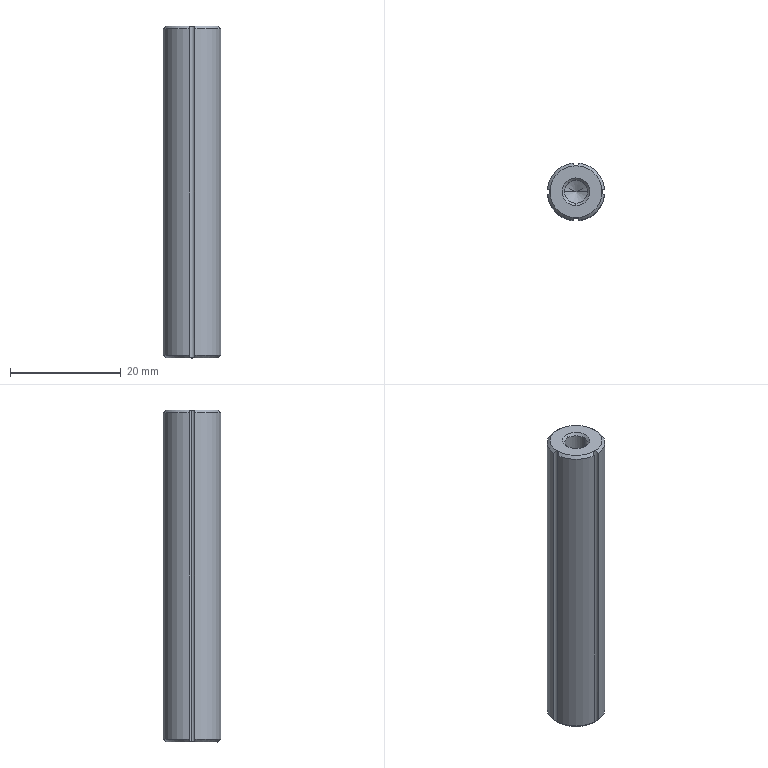Part | SolidWorks | features BaseBody 1 | 1 solid | 32 faces | box 10.348 x 10.348 x 60 mm | volume 4741 mm3 | cylinder 15 | cone 14 | plane 3 | commonest cylinder face diameters 1.04 x5 10.4 x4 2 x2 2.5 x2 4.134 x2
STEP:
#1=CARTESIAN_POINT('',(-4.68,0.,-30.));
#2=VERTEX_POINT('',#1);
#3=CARTESIAN_POINT('',(-4.698,0.1358,-30.));
#4=VERTEX_POINT('',#3);
#5=CARTESIAN_POINT('',(-5.2,0.,-30.));
#6=DIRECTION('',(0.,0.,1.));
#7=DIRECTION('',(1.,0.,0.));
#8=AXIS2_PLACEMENT_3D('',#5,#6,#7);
#9=CIRCLE('',#8,0.52);
#10=EDGE_CURVE('',#2,#4,#9,.T.);
#11=ORIENTED_EDGE('',*,*,#10,.F.);
#12=CARTESIAN_POINT('',(-4.68,0.,30.));
#13=VERTEX_POINT('',#12);
#14=CARTESIAN_POINT('',(-4.68,0.,30.));
#15=DIRECTION('',(0.,0.,1.));
#16=VECTOR('',#15,1000.);
#17=LINE('',#14,#16);
#18=EDGE_CURVE('',#2,#13,#17,.T.);
#19=ORIENTED_EDGE('',*,*,#18,.T.);
#20=CARTESIAN_POINT('',(-4.698,0.1358,30.));
#21=VERTEX_POINT('',#20);
#22=CARTESIAN_POINT('',(-5.2,0.,30.));
#23=DIRECTION('',(0.,0.,-1.));
#24=DIRECTION('',(1.,0.,0.));
#25=AXIS2_PLACEMENT_3D('',#22,#23,#24);
#26=CIRCLE('',#25,0.52);
#27=EDGE_CURVE('',#21,#13,#26,.T.);
#28=ORIENTED_EDGE('',*,*,#27,.F.);
#29=CARTESIAN_POINT('',(-5.174,0.5193,29.5));
#30=VERTEX_POINT('',#29);
#31=CARTESIAN_POINT('',(-5.174,0.5193,29.5));
#32=CARTESIAN_POINT('',(-5.076,0.5144,29.598));
#33=CARTESIAN_POINT('',(-4.981,0.483,29.696));
#34=CARTESIAN_POINT('',(-4.853,0.3908,29.831));
#35=CARTESIAN_POINT('',(-4.813,0.3523,29.874));
#36=CARTESIAN_POINT('',(-4.744,0.2574,29.949));
#37=CARTESIAN_POINT('',(-4.716,0.2008,29.981));
#38=CARTESIAN_POINT('',(-4.698,0.1358,30.));
#39=B_SPLINE_CURVE_WITH_KNOTS('',3,(#31,#32,#33,#34,#35,#36,#37,#38),.UNSPECIFIED.,.F.,.F.,(4,2,2,4),(0.,0.0004119,0.0006179,0.0008238),.UNSPECIFIED.);
#40=EDGE_CURVE('',#30,#21,#39,.T.);
#41=ORIENTED_EDGE('',*,*,#40,.F.);
#42=CARTESIAN_POINT('',(-5.174,0.5193,-29.5));
#43=VERTEX_POINT('',#42);
#44=CARTESIAN_POINT('',(-5.174,0.5193,0.));
#45=DIRECTION('',(0.,0.,1.));
#46=VECTOR('',#45,1000.);
#47=LINE('',#44,#46);
#48=EDGE_CURVE('',#43,#30,#47,.T.);
#49=ORIENTED_EDGE('',*,*,#48,.F.);
#50=CARTESIAN_POINT('',(-4.698,0.1358,-30.));
#51=CARTESIAN_POINT('',(-4.716,0.201,-29.98));
#52=CARTESIAN_POINT('',(-4.744,0.257,-29.949));
#53=CARTESIAN_POINT('',(-4.813,0.3519,-29.875));
#54=CARTESIAN_POINT('',(-4.852,0.3903,-29.832));
#55=CARTESIAN_POINT('',(-4.98,0.483,-29.696));
#56=CARTESIAN_POINT('',(-5.076,0.5144,-29.598));
#57=CARTESIAN_POINT('',(-5.174,0.5193,-29.5));
#58=B_SPLINE_CURVE_WITH_KNOTS('',3,(#50,#51,#52,#53,#54,#55,#56,#57),.UNSPECIFIED.,.F.,.F.,(4,2,2,4),(0.,0.0002068,0.0004137,0.0008273),.UNSPECIFIED.);
#59=EDGE_CURVE('',#4,#43,#58,.T.);
#60=ORIENTED_EDGE('',*,*,#59,.F.);
#61=EDGE_LOOP('',(#11,#19,#28,#41,#49,#60));
#62=FACE_OUTER_BOUND('',#61,.T.);
#63=CARTESIAN_POINT('',(-5.2,0.,30.));
#64=DIRECTION('',(0.,0.,1.));
#65=DIRECTION('',(1.,0.,0.));
#66=AXIS2_PLACEMENT_3D('',#63,#64,#65);
#67=CYLINDRICAL_SURFACE('',#66,0.52);
#68=ADVANCED_FACE('',(#62),#67,.F.);
#69=CARTESIAN_POINT('',(1.25,2.5,-22.5));
#70=VERTEX_POINT('',#69);
#71=CARTESIAN_POINT('',(-1.25,2.5,-22.5));
#72=VERTEX_POINT('',#71);
#73=CARTESIAN_POINT('',(0.,2.5,-22.5));
#74=DIRECTION('',(0.,0.,-1.));
#75=DIRECTION('',(-1.,0.,0.));
#76=AXIS2_PLACEMENT_3D('',#73,#74,#75);
#77=CIRCLE('',#76,1.25);
#78=EDGE_CURVE('',#70,#72,#77,.T.);
#79=ORIENTED_EDGE('',*,*,#78,.F.);
#80=CARTESIAN_POINT('',(1.25,2.5,-30.));
#81=VERTEX_POINT('',#80);
#82=CARTESIAN_POINT('',(1.25,2.5,-30.));
#83=DIRECTION('',(0.,0.,-1.));
#84=VECTOR('',#83,1000.);
#85=LINE('',#82,#84);
#86=EDGE_CURVE('',#70,#81,#85,.T.);
#87=ORIENTED_EDGE('',*,*,#86,.T.);
#88=CARTESIAN_POINT('',(-1.25,2.5,-30.));
#89=VERTEX_POINT('',#88);
#90=CARTESIAN_POINT('',(0.,2.5,-30.));
#91=DIRECTION('',(0.,0.,1.));
#92=DIRECTION('',(-1.,0.,0.));
#93=AXIS2_PLACEMENT_3D('',#90,#91,#92);
#94=CIRCLE('',#93,1.25);
#95=EDGE_CURVE('',#89,#81,#94,.T.);
#96=ORIENTED_EDGE('',*,*,#95,.F.);
#97=CARTESIAN_POINT('',(-1.25,2.5,-30.));
#98=DIRECTION('',(0.,0.,-1.));
#99=VECTOR('',#98,1000.);
#100=LINE('',#97,#99);
#101=EDGE_CURVE('',#72,#89,#100,.T.);
#102=ORIENTED_EDGE('',*,*,#101,.F.);
#103=EDGE_LOOP('',(#79,#87,#96,#102));
#104=FACE_OUTER_BOUND('',#103,.T.);
#105=CARTESIAN_POINT('',(0.,2.5,-30.));
#106=DIRECTION('',(0.,0.,-1.));
#107=DIRECTION('',(-1.,0.,0.));
#108=AXIS2_PLACEMENT_3D('',#105,#106,#107);
#109=CYLINDRICAL_SURFACE('',#108,1.25);
#110=ADVANCED_FACE('',(#104),#109,.F.);
#111=CARTESIAN_POINT('',(1.,-3.,-24.));
#112=VERTEX_POINT('',#111);
#113=CARTESIAN_POINT('',(-1.,-3.,-24.));
#114=VERTEX_POINT('',#113);
#115=CARTESIAN_POINT('',(0.,-3.,-24.));
#116=DIRECTION('',(0.,0.,-1.));
#117=DIRECTION('',(-1.,0.,0.));
#118=AXIS2_PLACEMENT_3D('',#115,#116,#117);
#119=CIRCLE('',#118,1.);
#120=EDGE_CURVE('',#112,#114,#119,.T.);
#121=ORIENTED_EDGE('',*,*,#120,.F.);
#122=CARTESIAN_POINT('',(1.,-3.,-30.));
#123=VERTEX_POINT('',#122);
#124=CARTESIAN_POINT('',(1.,-3.,-24.));
#125=DIRECTION('',(0.,0.,-1.));
#126=VECTOR('',#125,1000.);
#127=LINE('',#124,#126);
#128=EDGE_CURVE('',#112,#123,#127,.T.);
#129=ORIENTED_EDGE('',*,*,#128,.T.);
#130=CARTESIAN_POINT('',(-1.,-3.,-30.));
#131=VERTEX_POINT('',#130);
#132=CARTESIAN_POINT('',(0.,-3.,-30.));
#133=DIRECTION('',(0.,0.,1.));
#134=DIRECTION('',(-1.,0.,0.));
#135=AXIS2_PLACEMENT_3D('',#132,#133,#134);
#136=CIRCLE('',#135,1.);
#137=EDGE_CURVE('',#131,#123,#136,.T.);
#138=ORIENTED_EDGE('',*,*,#137,.F.);
#139=CARTESIAN_POINT('',(-1.,-3.,-24.));
#140=DIRECTION('',(0.,0.,-1.));
#141=VECTOR('',#140,1000.);
#142=LINE('',#139,#141);
#143=EDGE_CURVE('',#114,#131,#142,.T.);
#144=ORIENTED_EDGE('',*,*,#143,.F.);
#145=EDGE_LOOP('',(#121,#129,#138,#144));
#146=FACE_OUTER_BOUND('',#145,.T.);
#147=CARTESIAN_POINT('',(0.,-3.,-24.));
#148=DIRECTION('',(0.,0.,-1.));
#149=DIRECTION('',(-1.,0.,0.));
#150=AXIS2_PLACEMENT_3D('',#147,#148,#149);
#151=CYLINDRICAL_SURFACE('',#150,1.);
#152=ADVANCED_FACE('',(#146),#151,.F.);
#153=CARTESIAN_POINT('',(0.,2.067,29.567));
#154=VERTEX_POINT('',#153);
#155=CARTESIAN_POINT('',(-2.067,0.,29.567));
#156=VERTEX_POINT('',#155);
#157=CARTESIAN_POINT('',(0.,0.,29.567));
#158=DIRECTION('',(0.,0.,1.));
#159=DIRECTION('',(1.,0.,0.));
#160=AXIS2_PLACEMENT_3D('',#157,#158,#159);
#161=CIRCLE('',#160,2.067);
#162=EDGE_CURVE('',#154,#156,#161,.T.);
#163=ORIENTED_EDGE('',*,*,#162,.F.);
#164=CARTESIAN_POINT('',(0.,2.5,30.));
#165=VERTEX_POINT('',#164);
#166=CARTESIAN_POINT('',(0.,2.5,30.));
#167=DIRECTION('',(0.,0.7071,0.7071));
#168=VECTOR('',#167,1000.);
#169=LINE('',#166,#168);
#170=EDGE_CURVE('',#154,#165,#169,.T.);
#171=ORIENTED_EDGE('',*,*,#170,.T.);
#172=CARTESIAN_POINT('',(0.,-2.5,30.));
#173=VERTEX_POINT('',#172);
#174=CARTESIAN_POINT('',(0.,0.,30.));
#175=DIRECTION('',(0.,0.,-1.));
#176=DIRECTION('',(0.,-1.,0.));
#177=AXIS2_PLACEMENT_3D('',#174,#175,#176);
#178=CIRCLE('',#177,2.5);
#179=EDGE_CURVE('',#173,#165,#178,.T.);
#180=ORIENTED_EDGE('',*,*,#179,.F.);
#181=CARTESIAN_POINT('',(0.,-2.067,29.567));
#182=VERTEX_POINT('',#181);
#183=CARTESIAN_POINT('',(0.,-2.5,30.));
#184=DIRECTION('',(0.,-0.7071,0.7071));
#185=VECTOR('',#184,1000.);
#186=LINE('',#183,#185);
#187=EDGE_CURVE('',#182,#173,#186,.T.);
#188=ORIENTED_EDGE('',*,*,#187,.F.);
#189=CARTESIAN_POINT('',(0.,0.,29.567));
#190=DIRECTION('',(0.,0.,1.));
#191=DIRECTION('',(1.,0.,0.));
#192=AXIS2_PLACEMENT_3D('',#189,#190,#191);
#193=CIRCLE('',#192,2.067);
#194=EDGE_CURVE('',#156,#182,#193,.T.);
#195=ORIENTED_EDGE('',*,*,#194,.F.);
#196=EDGE_LOOP('',(#163,#171,#180,#188,#195));
#197=FACE_OUTER_BOUND('',#196,.T.);
#198=CARTESIAN_POINT('',(0.,0.,30.));
#199=DIRECTION('',(0.,0.,1.));
#200=DIRECTION('',(0.,-1.,0.));
#201=AXIS2_PLACEMENT_3D('',#198,#199,#200);
#202=CONICAL_SURFACE('',#201,2.5,0.7854);
#203=ADVANCED_FACE('',(#197),#202,.F.);
#204=CARTESIAN_POINT('',(0.,2.5,-21.749));
#205=VERTEX_POINT('',#204);
#206=CARTESIAN_POINT('',(-1.25,2.5,-22.5));
#207=DIRECTION('',(-0.8572,0.,-0.515));
#208=VECTOR('',#207,1000.);
#209=LINE('',#206,#208);
#210=EDGE_CURVE('',#205,#72,#209,.T.);
#211=ORIENTED_EDGE('',*,*,#210,.F.);
#212=CARTESIAN_POINT('',(1.25,2.5,-22.5));
#213=DIRECTION('',(0.8572,0.,-0.515));
#214=VECTOR('',#213,1000.);
#215=LINE('',#212,#214);
#216=EDGE_CURVE('',#205,#70,#215,.T.);
#217=ORIENTED_EDGE('',*,*,#216,.T.);
#218=ORIENTED_EDGE('',*,*,#78,.T.);
#219=EDGE_LOOP('',(#211,#217,#218));
#220=FACE_OUTER_BOUND('',#219,.T.);
#221=CARTESIAN_POINT('',(0.,2.5,-22.5));
#222=DIRECTION('',(0.,0.,-1.));
#223=DIRECTION('',(-1.,0.,0.));
#224=AXIS2_PLACEMENT_3D('',#221,#222,#223);
#225=CONICAL_SURFACE('',#224,1.25,1.03);
#226=ADVANCED_FACE('',(#220),#225,.F.);
#227=ORIENTED_EDGE('',*,*,#194,.T.);
#228=CARTESIAN_POINT('',(2.067,0.,29.567));
#229=VERTEX_POINT('',#228);
#230=CARTESIAN_POINT('',(0.,0.,29.567));
#231=DIRECTION('',(0.,0.,1.));
#232=DIRECTION('',(1.,0.,0.));
#233=AXIS2_PLACEMENT_3D('',#230,#231,#232);
#234=CIRCLE('',#233,2.067);
#235=EDGE_CURVE('',#182,#229,#234,.T.);
#236=ORIENTED_EDGE('',*,*,#235,.T.);
#237=CARTESIAN_POINT('',(2.067,0.,16.193));
#238=VERTEX_POINT('',#237);
#239=CARTESIAN_POINT('',(2.067,0.,22.88));
#240=DIRECTION('',(0.,0.,-1.));
#241=VECTOR('',#240,1000.);
#242=LINE('',#239,#241);
#243=EDGE_CURVE('',#229,#238,#242,.T.);
#244=ORIENTED_EDGE('',*,*,#243,.T.);
#245=CARTESIAN_POINT('',(-2.067,0.,16.193));
#246=VERTEX_POINT('',#245);
#247=CARTESIAN_POINT('',(0.,0.,16.193));
#248=DIRECTION('',(0.,0.,1.));
#249=DIRECTION('',(-1.,0.,0.));
#250=AXIS2_PLACEMENT_3D('',#247,#248,#249);
#251=CIRCLE('',#250,2.067);
#252=EDGE_CURVE('',#246,#238,#251,.T.);
#253=ORIENTED_EDGE('',*,*,#252,.F.);
#254=CARTESIAN_POINT('',(-2.067,0.,22.88));
#255=DIRECTION('',(0.,0.,-1.));
#256=VECTOR('',#255,1000.);
#257=LINE('',#254,#256);
#258=EDGE_CURVE('',#156,#246,#257,.T.);
#259=ORIENTED_EDGE('',*,*,#258,.F.);
#260=EDGE_LOOP('',(#227,#236,#244,#253,#259));
#261=FACE_OUTER_BOUND('',#260,.T.);
#262=CARTESIAN_POINT('',(0.,0.,22.88));
#263=DIRECTION('',(0.,0.,-1.));
#264=DIRECTION('',(-1.,0.,0.));
#265=AXIS2_PLACEMENT_3D('',#262,#263,#264);
#266=CYLINDRICAL_SURFACE('',#265,2.067);
#267=ADVANCED_FACE('',(#261),#266,.F.);
#268=CARTESIAN_POINT('',(0.,0.,15.));
#269=VERTEX_POINT('',#268);
#270=CARTESIAN_POINT('',(2.067,0.,16.193));
#271=DIRECTION('',(0.866,0.,0.5));
#272=VECTOR('',#271,1000.);
#273=LINE('',#270,#272);
#274=EDGE_CURVE('',#269,#238,#273,.T.);
#275=ORIENTED_EDGE('',*,*,#274,.F.);
#276=CARTESIAN_POINT('',(-2.067,0.,16.193));
#277=DIRECTION('',(-0.866,0.,0.5));
#278=VECTOR('',#277,1000.);
#279=LINE('',#276,#278);
#280=EDGE_CURVE('',#269,#246,#279,.T.);
#281=ORIENTED_EDGE('',*,*,#280,.T.);
#282=ORIENTED_EDGE('',*,*,#252,.T.);
#283=EDGE_LOOP('',(#275,#281,#282));
#284=FACE_OUTER_BOUND('',#283,.T.);
#285=CARTESIAN_POINT('',(0.,0.,16.193));
#286=DIRECTION('',(0.,0.,1.));
#287=DIRECTION('',(1.,0.,0.));
#288=AXIS2_PLACEMENT_3D('',#285,#286,#287);
#289=CONICAL_SURFACE('',#288,2.067,1.047);
#290=ADVANCED_FACE('',(#284),#289,.F.);
#291=CARTESIAN_POINT('',(-0.5193,5.174,29.5));
#292=VERTEX_POINT('',#291);
#293=CARTESIAN_POINT('',(-0.5193,5.174,-29.5));
#294=VERTEX_POINT('',#293);
#295=CARTESIAN_POINT('',(-0.5193,5.174,0.));
#296=DIRECTION('',(0.,0.,-1.));
#297=VECTOR('',#296,1000.);
#298=LINE('',#295,#297);
#299=EDGE_CURVE('',#292,#294,#298,.T.);
#300=ORIENTED_EDGE('',*,*,#299,.T.);
#301=CARTESIAN_POINT('',(0.,0.,-29.5));
#302=DIRECTION('',(0.,0.,1.));
#303=DIRECTION('',(-1.,0.,0.));
#304=AXIS2_PLACEMENT_3D('',#301,#302,#303);
#305=CIRCLE('',#304,5.2);
#306=EDGE_CURVE('',#294,#43,#305,.T.);
#307=ORIENTED_EDGE('',*,*,#306,.T.);
#308=ORIENTED_EDGE('',*,*,#48,.T.);
#309=CARTESIAN_POINT('',(0.,0.,29.5));
#310=DIRECTION('',(0.,0.,-1.));
#311=DIRECTION('',(-1.,0.,0.));
#312=AXIS2_PLACEMENT_3D('',#309,#310,#311);
#313=CIRCLE('',#312,5.2);
#314=EDGE_CURVE('',#30,#292,#313,.T.);
#315=ORIENTED_EDGE('',*,*,#314,.T.);
#316=EDGE_LOOP('',(#300,#307,#308,#315));
#317=FACE_OUTER_BOUND('',#316,.T.);
#318=CARTESIAN_POINT('',(0.,0.,0.));
#319=DIRECTION('',(0.,0.,-1.));
#320=DIRECTION('',(-1.,0.,0.));
#321=AXIS2_PLACEMENT_3D('',#318,#319,#320);
#322=CYLINDRICAL_SURFACE('',#321,5.2);
#323=ADVANCED_FACE('',(#317),#322,.T.);
#324=CARTESIAN_POINT('',(-0.1358,4.698,-30.));
#325=VERTEX_POINT('',#324);
#326=CARTESIAN_POINT('',(-0.5193,5.174,-29.5));
#327=CARTESIAN_POINT('',(-0.5144,5.076,-29.598));
#328=CARTESIAN_POINT('',(-0.483,4.981,-29.696));
#329=CARTESIAN_POINT('',(-0.3908,4.853,-29.831));
#330=CARTESIAN_POINT('',(-0.3523,4.813,-29.874));
#331=CARTESIAN_POINT('',(-0.2574,4.744,-29.949));
#332=CARTESIAN_POINT('',(-0.2008,4.716,-29.981));
#333=CARTESIAN_POINT('',(-0.1358,4.698,-30.));
#334=B_SPLINE_CURVE_WITH_KNOTS('',3,(#326,#327,#328,#329,#330,#331,#332,#333),.UNSPECIFIED.,.F.,.F.,(4,2,2,4),(0.,0.0004119,0.0006179,0.0008238),.UNSPECIFIED.);
#335=EDGE_CURVE('',#294,#325,#334,.T.);
#336=ORIENTED_EDGE('',*,*,#335,.T.);
#337=CARTESIAN_POINT('',(0.,0.,-30.));
#338=DIRECTION('',(0.,0.,1.));
#339=DIRECTION('',(0.,-1.,0.));
#340=AXIS2_PLACEMENT_3D('',#337,#338,#339);
#341=CIRCLE('',#340,4.7);
#342=EDGE_CURVE('',#325,#4,#341,.T.);
#343=ORIENTED_EDGE('',*,*,#342,.T.);
#344=ORIENTED_EDGE('',*,*,#59,.T.);
#345=ORIENTED_EDGE('',*,*,#306,.F.);
#346=EDGE_LOOP('',(#336,#343,#344,#345));
#347=FACE_OUTER_BOUND('',#346,.T.);
#348=CARTESIAN_POINT('',(0.,0.,-29.5));
#349=DIRECTION('',(0.,0.,1.));
#350=DIRECTION('',(0.,-1.,0.));
#351=AXIS2_PLACEMENT_3D('',#348,#349,#350);
#352=CONICAL_SURFACE('',#351,5.2,0.7854);
#353=ADVANCED_FACE('',(#347),#352,.T.);
#354=CARTESIAN_POINT('',(0.1358,4.698,-30.));
#355=VERTEX_POINT('',#354);
#356=CARTESIAN_POINT('',(0.5193,5.174,-29.5));
#357=VERTEX_POINT('',#356);
#358=CARTESIAN_POINT('',(0.1358,4.698,-30.));
#359=CARTESIAN_POINT('',(0.201,4.716,-29.98));
#360=CARTESIAN_POINT('',(0.257,4.744,-29.949));
#361=CARTESIAN_POINT('',(0.3519,4.813,-29.875));
#362=CARTESIAN_POINT('',(0.3903,4.852,-29.832));
#363=CARTESIAN_POINT('',(0.483,4.98,-29.696));
#364=CARTESIAN_POINT('',(0.5144,5.076,-29.598));
#365=CARTESIAN_POINT('',(0.5193,5.174,-29.5));
#366=B_SPLINE_CURVE_WITH_KNOTS('',3,(#358,#359,#360,#361,#362,#363,#364,#365),.UNSPECIFIED.,.F.,.F.,(4,2,2,4),(0.,0.0002068,0.0004137,0.0008273),.UNSPECIFIED.);
#367=EDGE_CURVE('',#355,#357,#366,.T.);
#368=ORIENTED_EDGE('',*,*,#367,.F.);
#369=CARTESIAN_POINT('',(0.,5.2,-30.));
#370=DIRECTION('',(0.,0.,1.));
#371=DIRECTION('',(1.,0.,0.));
#372=AXIS2_PLACEMENT_3D('',#369,#370,#371);
#373=CIRCLE('',#372,0.52);
#374=EDGE_CURVE('',#325,#355,#373,.T.);
#375=ORIENTED_EDGE('',*,*,#374,.F.);
#376=ORIENTED_EDGE('',*,*,#335,.F.);
#377=ORIENTED_EDGE('',*,*,#299,.F.);
#378=CARTESIAN_POINT('',(-0.1358,4.698,30.));
#379=VERTEX_POINT('',#378);
#380=CARTESIAN_POINT('',(-0.1358,4.698,30.));
#381=CARTESIAN_POINT('',(-0.201,4.716,29.98));
#382=CARTESIAN_POINT('',(-0.257,4.744,29.949));
#383=CARTESIAN_POINT('',(-0.3519,4.813,29.875));
#384=CARTESIAN_POINT('',(-0.3903,4.852,29.832));
#385=CARTESIAN_POINT('',(-0.483,4.98,29.696));
#386=CARTESIAN_POINT('',(-0.5144,5.076,29.598));
#387=CARTESIAN_POINT('',(-0.5193,5.174,29.5));
#388=B_SPLINE_CURVE_WITH_KNOTS('',3,(#380,#381,#382,#383,#384,#385,#386,#387),.UNSPECIFIED.,.F.,.F.,(4,2,2,4),(0.,0.0002068,0.0004137,0.0008273),.UNSPECIFIED.);
#389=EDGE_CURVE('',#379,#292,#388,.T.);
#390=ORIENTED_EDGE('',*,*,#389,.F.);
#391=CARTESIAN_POINT('',(0.1358,4.698,30.));
#392=VERTEX_POINT('',#391);
#393=CARTESIAN_POINT('',(0.,5.2,30.));
#394=DIRECTION('',(0.,0.,-1.));
#395=DIRECTION('',(1.,0.,0.));
#396=AXIS2_PLACEMENT_3D('',#393,#394,#395);
#397=CIRCLE('',#396,0.52);
#398=EDGE_CURVE('',#392,#379,#397,.T.);
#399=ORIENTED_EDGE('',*,*,#398,.F.);
#400=CARTESIAN_POINT('',(0.5193,5.174,29.5));
#401=VERTEX_POINT('',#400);
#402=CARTESIAN_POINT('',(0.5193,5.174,29.5));
#403=CARTESIAN_POINT('',(0.5144,5.076,29.598));
#404=CARTESIAN_POINT('',(0.483,4.981,29.696));
#405=CARTESIAN_POINT('',(0.3908,4.853,29.831));
#406=CARTESIAN_POINT('',(0.3523,4.813,29.874));
#407=CARTESIAN_POINT('',(0.2574,4.744,29.949));
#408=CARTESIAN_POINT('',(0.2008,4.716,29.981));
#409=CARTESIAN_POINT('',(0.1358,4.698,30.));
#410=B_SPLINE_CURVE_WITH_KNOTS('',3,(#402,#403,#404,#405,#406,#407,#408,#409),.UNSPECIFIED.,.F.,.F.,(4,2,2,4),(0.,0.0004119,0.0006179,0.0008238),.UNSPECIFIED.);
#411=EDGE_CURVE('',#401,#392,#410,.T.);
#412=ORIENTED_EDGE('',*,*,#411,.F.);
#413=CARTESIAN_POINT('',(0.5193,5.174,30.));
#414=DIRECTION('',(0.,0.,1.));
#415=VECTOR('',#414,1000.);
#416=LINE('',#413,#415);
#417=EDGE_CURVE('',#357,#401,#416,.T.);
#418=ORIENTED_EDGE('',*,*,#417,.F.);
#419=EDGE_LOOP('',(#368,#375,#376,#377,#390,#399,#412,#418));
#420=FACE_OUTER_BOUND('',#419,.T.);
#421=CARTESIAN_POINT('',(0.,5.2,30.));
#422=DIRECTION('',(0.,0.,1.));
#423=DIRECTION('',(1.,0.,0.));
#424=AXIS2_PLACEMENT_3D('',#421,#422,#423);
#425=CYLINDRICAL_SURFACE('',#424,0.52);
#426=ADVANCED_FACE('',(#420),#425,.F.);
#427=ORIENTED_EDGE('',*,*,#389,.T.);
#428=ORIENTED_EDGE('',*,*,#314,.F.);
#429=ORIENTED_EDGE('',*,*,#40,.T.);
#430=CARTESIAN_POINT('',(0.,0.,30.));
#431=DIRECTION('',(0.,0.,-1.));
#432=DIRECTION('',(-1.,0.,0.));
#433=AXIS2_PLACEMENT_3D('',#430,#431,#432);
#434=CIRCLE('',#433,4.7);
#435=EDGE_CURVE('',#21,#379,#434,.T.);
#436=ORIENTED_EDGE('',*,*,#435,.T.);
#437=EDGE_LOOP('',(#427,#428,#429,#436));
#438=FACE_OUTER_BOUND('',#437,.T.);
#439=CARTESIAN_POINT('',(0.,0.,29.5));
#440=DIRECTION('',(0.,0.,-1.));
#441=DIRECTION('',(-1.,0.,0.));
#442=AXIS2_PLACEMENT_3D('',#439,#440,#441);
#443=CONICAL_SURFACE('',#442,5.2,0.7854);
#444=ADVANCED_FACE('',(#438),#443,.T.);
#445=ORIENTED_EDGE('',*,*,#18,.F.);
#446=CARTESIAN_POINT('',(-4.698,-0.1358,-30.));
#447=VERTEX_POINT('',#446);
#448=CARTESIAN_POINT('',(-5.2,0.,-30.));
#449=DIRECTION('',(0.,0.,1.));
#450=DIRECTION('',(1.,0.,0.));
#451=AXIS2_PLACEMENT_3D('',#448,#449,#450);
#452=CIRCLE('',#451,0.52);
#453=EDGE_CURVE('',#447,#2,#452,.T.);
#454=ORIENTED_EDGE('',*,*,#453,.F.);
#455=CARTESIAN_POINT('',(-5.174,-0.5193,-29.5));
#456=VERTEX_POINT('',#455);
#457=CARTESIAN_POINT('',(-5.174,-0.5193,-29.5));
#458=CARTESIAN_POINT('',(-5.076,-0.5144,-29.598));
#459=CARTESIAN_POINT('',(-4.981,-0.483,-29.696));
#460=CARTESIAN_POINT('',(-4.853,-0.3908,-29.831));
#461=CARTESIAN_POINT('',(-4.813,-0.3523,-29.874));
#462=CARTESIAN_POINT('',(-4.744,-0.2574,-29.949));
#463=CARTESIAN_POINT('',(-4.716,-0.2008,-29.981));
#464=CARTESIAN_POINT('',(-4.698,-0.1358,-30.));
#465=B_SPLINE_CURVE_WITH_KNOTS('',3,(#457,#458,#459,#460,#461,#462,#463,#464),.UNSPECIFIED.,.F.,.F.,(4,2,2,4),(0.,0.0004119,0.0006179,0.0008238),.UNSPECIFIED.);
#466=EDGE_CURVE('',#456,#447,#465,.T.);
#467=ORIENTED_EDGE('',*,*,#466,.F.);
#468=CARTESIAN_POINT('',(-5.174,-0.5193,29.5));
#469=VERTEX_POINT('',#468);
#470=CARTESIAN_POINT('',(-5.174,-0.5193,30.));
#471=DIRECTION('',(0.,0.,-1.));
#472=VECTOR('',#471,1000.);
#473=LINE('',#470,#472);
#474=EDGE_CURVE('',#469,#456,#473,.T.);
#475=ORIENTED_EDGE('',*,*,#474,.F.);
#476=CARTESIAN_POINT('',(-4.698,-0.1358,30.));
#477=VERTEX_POINT('',#476);
#478=CARTESIAN_POINT('',(-4.698,-0.1358,30.));
#479=CARTESIAN_POINT('',(-4.716,-0.201,29.98));
#480=CARTESIAN_POINT('',(-4.744,-0.257,29.949));
#481=CARTESIAN_POINT('',(-4.813,-0.3519,29.875));
#482=CARTESIAN_POINT('',(-4.852,-0.3903,29.832));
#483=CARTESIAN_POINT('',(-4.98,-0.483,29.696));
#484=CARTESIAN_POINT('',(-5.076,-0.5144,29.598));
#485=CARTESIAN_POINT('',(-5.174,-0.5193,29.5));
#486=B_SPLINE_CURVE_WITH_KNOTS('',3,(#478,#479,#480,#481,#482,#483,#484,#485),.UNSPECIFIED.,.F.,.F.,(4,2,2,4),(0.,0.0002068,0.0004137,0.0008273),.UNSPECIFIED.);
#487=EDGE_CURVE('',#477,#469,#486,.T.);
#488=ORIENTED_EDGE('',*,*,#487,.F.);
#489=CARTESIAN_POINT('',(-5.2,0.,30.));
#490=DIRECTION('',(0.,0.,-1.));
#491=DIRECTION('',(1.,0.,0.));
#492=AXIS2_PLACEMENT_3D('',#489,#490,#491);
#493=CIRCLE('',#492,0.52);
#494=EDGE_CURVE('',#13,#477,#493,.T.);
#495=ORIENTED_EDGE('',*,*,#494,.F.);
#496=EDGE_LOOP('',(#445,#454,#467,#475,#488,#495));
#497=FACE_OUTER_BOUND('',#496,.T.);
#498=CARTESIAN_POINT('',(-5.2,0.,30.));
#499=DIRECTION('',(0.,0.,1.));
#500=DIRECTION('',(1.,0.,0.));
#501=AXIS2_PLACEMENT_3D('',#498,#499,#500);
#502=CYLINDRICAL_SURFACE('',#501,0.52);
#503=ADVANCED_FACE('',(#497),#502,.F.);
#504=ORIENTED_EDGE('',*,*,#453,.T.);
#505=ORIENTED_EDGE('',*,*,#10,.T.);
#506=ORIENTED_EDGE('',*,*,#342,.F.);
#507=ORIENTED_EDGE('',*,*,#374,.T.);
#508=CARTESIAN_POINT('',(4.698,0.1358,-30.));
#509=VERTEX_POINT('',#508);
#510=CARTESIAN_POINT('',(0.,0.,-30.));
#511=DIRECTION('',(0.,0.,-1.));
#512=DIRECTION('',(0.,-1.,0.));
#513=AXIS2_PLACEMENT_3D('',#510,#511,#512);
#514=CIRCLE('',#513,4.7);
#515=EDGE_CURVE('',#355,#509,#514,.T.);
#516=ORIENTED_EDGE('',*,*,#515,.T.);
#517=CARTESIAN_POINT('',(4.698,-0.1358,-30.));
#518=VERTEX_POINT('',#517);
#519=CARTESIAN_POINT('',(5.2,0.,-30.));
#520=DIRECTION('',(0.,0.,1.));
#521=DIRECTION('',(1.,0.,0.));
#522=AXIS2_PLACEMENT_3D('',#519,#520,#521);
#523=CIRCLE('',#522,0.52);
#524=EDGE_CURVE('',#509,#518,#523,.T.);
#525=ORIENTED_EDGE('',*,*,#524,.T.);
#526=CARTESIAN_POINT('',(0.1358,-4.698,-30.));
#527=VERTEX_POINT('',#526);
#528=CARTESIAN_POINT('',(0.,0.,-30.));
#529=DIRECTION('',(0.,0.,-1.));
#530=DIRECTION('',(0.,-1.,0.));
#531=AXIS2_PLACEMENT_3D('',#528,#529,#530);
#532=CIRCLE('',#531,4.7);
#533=EDGE_CURVE('',#518,#527,#532,.T.);
#534=ORIENTED_EDGE('',*,*,#533,.T.);
#535=CARTESIAN_POINT('',(-0.1358,-4.698,-30.));
#536=VERTEX_POINT('',#535);
#537=CARTESIAN_POINT('',(0.,-5.2,-30.));
#538=DIRECTION('',(0.,0.,1.));
#539=DIRECTION('',(1.,0.,0.));
#540=AXIS2_PLACEMENT_3D('',#537,#538,#539);
#541=CIRCLE('',#540,0.52);
#542=EDGE_CURVE('',#527,#536,#541,.T.);
#543=ORIENTED_EDGE('',*,*,#542,.T.);
#544=CARTESIAN_POINT('',(0.,0.,-30.));
#545=DIRECTION('',(0.,0.,-1.));
#546=DIRECTION('',(0.,-1.,0.));
#547=AXIS2_PLACEMENT_3D('',#544,#545,#546);
#548=CIRCLE('',#547,4.7);
#549=EDGE_CURVE('',#536,#447,#548,.T.);
#550=ORIENTED_EDGE('',*,*,#549,.T.);
#551=EDGE_LOOP('',(#504,#505,#506,#507,#516,#525,#534,#543,#550));
#552=FACE_OUTER_BOUND('',#551,.T.);
#553=ORIENTED_EDGE('',*,*,#95,.T.);
#554=CARTESIAN_POINT('',(0.,2.5,-30.));
#555=DIRECTION('',(0.,0.,1.));
#556=DIRECTION('',(-1.,0.,0.));
#557=AXIS2_PLACEMENT_3D('',#554,#555,#556);
#558=CIRCLE('',#557,1.25);
#559=EDGE_CURVE('',#81,#89,#558,.T.);
#560=ORIENTED_EDGE('',*,*,#559,.T.);
#561=EDGE_LOOP('',(#553,#560));
#562=FACE_BOUND('',#561,.T.);
#563=ORIENTED_EDGE('',*,*,#137,.T.);
#564=CARTESIAN_POINT('',(0.,-3.,-30.));
#565=DIRECTION('',(0.,0.,1.));
#566=DIRECTION('',(-1.,0.,0.));
#567=AXIS2_PLACEMENT_3D('',#564,#565,#566);
#568=CIRCLE('',#567,1.);
#569=EDGE_CURVE('',#123,#131,#568,.T.);
#570=ORIENTED_EDGE('',*,*,#569,.T.);
#571=EDGE_LOOP('',(#563,#570));
#572=FACE_BOUND('',#571,.T.);
#573=CARTESIAN_POINT('',(0.,2.35,-30.));
#574=DIRECTION('',(0.,0.,-1.));
#575=DIRECTION('',(-1.,0.,0.));
#576=AXIS2_PLACEMENT_3D('',#573,#574,#575);
#577=PLANE('',#576);
#578=ADVANCED_FACE('',(#552,#562,#572),#577,.T.);
#579=CARTESIAN_POINT('',(5.174,0.5193,29.5));
#580=VERTEX_POINT('',#579);
#581=CARTESIAN_POINT('',(5.174,0.5193,-29.5));
#582=VERTEX_POINT('',#581);
#583=CARTESIAN_POINT('',(5.174,0.5193,0.));
#584=DIRECTION('',(0.,0.,-1.));
#585=VECTOR('',#584,1000.);
#586=LINE('',#583,#585);
#587=EDGE_CURVE('',#580,#582,#586,.T.);
#588=ORIENTED_EDGE('',*,*,#587,.T.);
#589=CARTESIAN_POINT('',(0.,0.,-29.5));
#590=DIRECTION('',(0.,0.,1.));
#591=DIRECTION('',(-1.,0.,0.));
#592=AXIS2_PLACEMENT_3D('',#589,#590,#591);
#593=CIRCLE('',#592,5.2);
#594=EDGE_CURVE('',#582,#357,#593,.T.);
#595=ORIENTED_EDGE('',*,*,#594,.T.);
#596=ORIENTED_EDGE('',*,*,#417,.T.);
#597=CARTESIAN_POINT('',(0.,0.,29.5));
#598=DIRECTION('',(0.,0.,-1.));
#599=DIRECTION('',(-1.,0.,0.));
#600=AXIS2_PLACEMENT_3D('',#597,#598,#599);
#601=CIRCLE('',#600,5.2);
#602=EDGE_CURVE('',#401,#580,#601,.T.);
#603=ORIENTED_EDGE('',*,*,#602,.T.);
#604=EDGE_LOOP('',(#588,#595,#596,#603));
#605=FACE_OUTER_BOUND('',#604,.T.);
#606=CARTESIAN_POINT('',(0.,0.,0.));
#607=DIRECTION('',(0.,0.,-1.));
#608=DIRECTION('',(-1.,0.,0.));
#609=AXIS2_PLACEMENT_3D('',#606,#607,#608);
#610=CYLINDRICAL_SURFACE('',#609,5.2);
#611=ADVANCED_FACE('',(#605),#610,.T.);
#612=ORIENTED_EDGE('',*,*,#27,.T.);
#613=ORIENTED_EDGE('',*,*,#494,.T.);
#614=CARTESIAN_POINT('',(-0.1358,-4.698,30.));
#615=VERTEX_POINT('',#614);
#616=CARTESIAN_POINT('',(0.,0.,30.));
#617=DIRECTION('',(0.,0.,1.));
#618=DIRECTION('',(0.,1.,0.));
#619=AXIS2_PLACEMENT_3D('',#616,#617,#618);
#620=CIRCLE('',#619,4.7);
#621=EDGE_CURVE('',#477,#615,#620,.T.);
#622=ORIENTED_EDGE('',*,*,#621,.T.);
#623=CARTESIAN_POINT('',(0.1358,-4.698,30.));
#624=VERTEX_POINT('',#623);
#625=CARTESIAN_POINT('',(0.,-5.2,30.));
#626=DIRECTION('',(0.,0.,-1.));
#627=DIRECTION('',(1.,0.,0.));
#628=AXIS2_PLACEMENT_3D('',#625,#626,#627);
#629=CIRCLE('',#628,0.52);
#630=EDGE_CURVE('',#615,#624,#629,.T.);
#631=ORIENTED_EDGE('',*,*,#630,.T.);
#632=CARTESIAN_POINT('',(4.698,-0.1358,30.));
#633=VERTEX_POINT('',#632);
#634=CARTESIAN_POINT('',(0.,0.,30.));
#635=DIRECTION('',(0.,0.,1.));
#636=DIRECTION('',(0.,1.,0.));
#637=AXIS2_PLACEMENT_3D('',#634,#635,#636);
#638=CIRCLE('',#637,4.7);
#639=EDGE_CURVE('',#624,#633,#638,.T.);
#640=ORIENTED_EDGE('',*,*,#639,.T.);
#641=CARTESIAN_POINT('',(4.698,0.1358,30.));
#642=VERTEX_POINT('',#641);
#643=CARTESIAN_POINT('',(5.2,0.,30.));
#644=DIRECTION('',(0.,0.,-1.));
#645=DIRECTION('',(1.,0.,0.));
#646=AXIS2_PLACEMENT_3D('',#643,#644,#645);
#647=CIRCLE('',#646,0.52);
#648=EDGE_CURVE('',#633,#642,#647,.T.);
#649=ORIENTED_EDGE('',*,*,#648,.T.);
#650=CARTESIAN_POINT('',(0.,0.,30.));
#651=DIRECTION('',(0.,0.,1.));
#652=DIRECTION('',(0.,1.,0.));
#653=AXIS2_PLACEMENT_3D('',#650,#651,#652);
#654=CIRCLE('',#653,4.7);
#655=EDGE_CURVE('',#642,#392,#654,.T.);
#656=ORIENTED_EDGE('',*,*,#655,.T.);
#657=ORIENTED_EDGE('',*,*,#398,.T.);
#658=ORIENTED_EDGE('',*,*,#435,.F.);
#659=EDGE_LOOP('',(#612,#613,#622,#631,#640,#649,#656,#657,#658));
#660=FACE_OUTER_BOUND('',#659,.T.);
#661=ORIENTED_EDGE('',*,*,#179,.T.);
#662=CARTESIAN_POINT('',(0.,0.,30.));
#663=DIRECTION('',(0.,0.,-1.));
#664=DIRECTION('',(0.,-1.,0.));
#665=AXIS2_PLACEMENT_3D('',#662,#663,#664);
#666=CIRCLE('',#665,2.5);
#667=EDGE_CURVE('',#165,#173,#666,.T.);
#668=ORIENTED_EDGE('',*,*,#667,.T.);
#669=EDGE_LOOP('',(#661,#668));
#670=FACE_BOUND('',#669,.T.);
#671=CARTESIAN_POINT('',(0.,3.6,30.));
#672=DIRECTION('',(0.,0.,1.));
#673=DIRECTION('',(1.,0.,0.));
#674=AXIS2_PLACEMENT_3D('',#671,#672,#673);
#675=PLANE('',#674);
#676=ADVANCED_FACE('',(#660,#670),#675,.T.);
#677=CARTESIAN_POINT('',(-0.5193,-5.174,-29.5));
#678=VERTEX_POINT('',#677);
#679=CARTESIAN_POINT('',(-0.1358,-4.698,-30.));
#680=CARTESIAN_POINT('',(-0.201,-4.716,-29.98));
#681=CARTESIAN_POINT('',(-0.257,-4.744,-29.949));
#682=CARTESIAN_POINT('',(-0.3519,-4.813,-29.875));
#683=CARTESIAN_POINT('',(-0.3903,-4.852,-29.832));
#684=CARTESIAN_POINT('',(-0.483,-4.98,-29.696));
#685=CARTESIAN_POINT('',(-0.5144,-5.076,-29.598));
#686=CARTESIAN_POINT('',(-0.5193,-5.174,-29.5));
#687=B_SPLINE_CURVE_WITH_KNOTS('',3,(#679,#680,#681,#682,#683,#684,#685,#686),.UNSPECIFIED.,.F.,.F.,(4,2,2,4),(0.,0.0002068,0.0004137,0.0008273),.UNSPECIFIED.);
#688=EDGE_CURVE('',#536,#678,#687,.T.);
#689=ORIENTED_EDGE('',*,*,#688,.T.);
#690=CARTESIAN_POINT('',(0.,0.,-29.5));
#691=DIRECTION('',(0.,0.,-1.));
#692=DIRECTION('',(1.,0.,0.));
#693=AXIS2_PLACEMENT_3D('',#690,#691,#692);
#694=CIRCLE('',#693,5.2);
#695=EDGE_CURVE('',#678,#456,#694,.T.);
#696=ORIENTED_EDGE('',*,*,#695,.T.);
#697=ORIENTED_EDGE('',*,*,#466,.T.);
#698=ORIENTED_EDGE('',*,*,#549,.F.);
#699=EDGE_LOOP('',(#689,#696,#697,#698));
#700=FACE_OUTER_BOUND('',#699,.T.);
#701=CARTESIAN_POINT('',(0.,0.,-29.5));
#702=DIRECTION('',(0.,0.,1.));
#703=DIRECTION('',(0.,-1.,0.));
#704=AXIS2_PLACEMENT_3D('',#701,#702,#703);
#705=CONICAL_SURFACE('',#704,5.2,0.7854);
#706=ADVANCED_FACE('',(#700),#705,.T.);
#707=CARTESIAN_POINT('',(5.174,-0.5193,-29.5));
#708=VERTEX_POINT('',#707);
#709=CARTESIAN_POINT('',(4.698,-0.1358,-30.));
#710=CARTESIAN_POINT('',(4.716,-0.201,-29.98));
#711=CARTESIAN_POINT('',(4.744,-0.257,-29.949));
#712=CARTESIAN_POINT('',(4.813,-0.3519,-29.875));
#713=CARTESIAN_POINT('',(4.852,-0.3903,-29.832));
#714=CARTESIAN_POINT('',(4.98,-0.483,-29.696));
#715=CARTESIAN_POINT('',(5.076,-0.5144,-29.598));
#716=CARTESIAN_POINT('',(5.174,-0.5193,-29.5));
#717=B_SPLINE_CURVE_WITH_KNOTS('',3,(#709,#710,#711,#712,#713,#714,#715,#716),.UNSPECIFIED.,.F.,.F.,(4,2,2,4),(0.,0.0002068,0.0004137,0.0008273),.UNSPECIFIED.);
#718=EDGE_CURVE('',#518,#708,#717,.T.);
#719=ORIENTED_EDGE('',*,*,#718,.T.);
#720=CARTESIAN_POINT('',(0.5193,-5.174,-29.5));
#721=VERTEX_POINT('',#720);
#722=CARTESIAN_POINT('',(0.,0.,-29.5));
#723=DIRECTION('',(0.,0.,-1.));
#724=DIRECTION('',(1.,0.,0.));
#725=AXIS2_PLACEMENT_3D('',#722,#723,#724);
#726=CIRCLE('',#725,5.2);
#727=EDGE_CURVE('',#708,#721,#726,.T.);
#728=ORIENTED_EDGE('',*,*,#727,.T.);
#729=CARTESIAN_POINT('',(0.5193,-5.174,-29.5));
#730=CARTESIAN_POINT('',(0.5144,-5.076,-29.598));
#731=CARTESIAN_POINT('',(0.483,-4.981,-29.696));
#732=CARTESIAN_POINT('',(0.3908,-4.853,-29.831));
#733=CARTESIAN_POINT('',(0.3523,-4.813,-29.874));
#734=CARTESIAN_POINT('',(0.2574,-4.744,-29.949));
#735=CARTESIAN_POINT('',(0.2008,-4.716,-29.981));
#736=CARTESIAN_POINT('',(0.1358,-4.698,-30.));
#737=B_SPLINE_CURVE_WITH_KNOTS('',3,(#729,#730,#731,#732,#733,#734,#735,#736),.UNSPECIFIED.,.F.,.F.,(4,2,2,4),(0.,0.0004119,0.0006179,0.0008238),.UNSPECIFIED.);
#738=EDGE_CURVE('',#721,#527,#737,.T.);
#739=ORIENTED_EDGE('',*,*,#738,.T.);
#740=ORIENTED_EDGE('',*,*,#533,.F.);
#741=EDGE_LOOP('',(#719,#728,#739,#740));
#742=FACE_OUTER_BOUND('',#741,.T.);
#743=CARTESIAN_POINT('',(0.,0.,-29.5));
#744=DIRECTION('',(0.,0.,1.));
#745=DIRECTION('',(0.,-1.,0.));
#746=AXIS2_PLACEMENT_3D('',#743,#744,#745);
#747=CONICAL_SURFACE('',#746,5.2,0.7854);
#748=ADVANCED_FACE('',(#742),#747,.T.);
#749=CARTESIAN_POINT('',(5.174,0.5193,-29.5));
#750=CARTESIAN_POINT('',(5.076,0.5144,-29.598));
#751=CARTESIAN_POINT('',(4.981,0.483,-29.696));
#752=CARTESIAN_POINT('',(4.853,0.3908,-29.831));
#753=CARTESIAN_POINT('',(4.813,0.3523,-29.874));
#754=CARTESIAN_POINT('',(4.744,0.2574,-29.949));
#755=CARTESIAN_POINT('',(4.716,0.2008,-29.981));
#756=CARTESIAN_POINT('',(4.698,0.1358,-30.));
#757=B_SPLINE_CURVE_WITH_KNOTS('',3,(#749,#750,#751,#752,#753,#754,#755,#756),.UNSPECIFIED.,.F.,.F.,(4,2,2,4),(0.,0.0004119,0.0006179,0.0008238),.UNSPECIFIED.);
#758=EDGE_CURVE('',#582,#509,#757,.T.);
#759=ORIENTED_EDGE('',*,*,#758,.T.);
#760=ORIENTED_EDGE('',*,*,#515,.F.);
#761=ORIENTED_EDGE('',*,*,#367,.T.);
#762=ORIENTED_EDGE('',*,*,#594,.F.);
#763=EDGE_LOOP('',(#759,#760,#761,#762));
#764=FACE_OUTER_BOUND('',#763,.T.);
#765=CARTESIAN_POINT('',(0.,0.,-29.5));
#766=DIRECTION('',(0.,0.,1.));
#767=DIRECTION('',(0.,-1.,0.));
#768=AXIS2_PLACEMENT_3D('',#765,#766,#767);
#769=CONICAL_SURFACE('',#768,5.2,0.7854);
#770=ADVANCED_FACE('',(#764),#769,.T.);
#771=ORIENTED_EDGE('',*,*,#86,.F.);
#772=CARTESIAN_POINT('',(0.,2.5,-22.5));
#773=DIRECTION('',(0.,0.,-1.));
#774=DIRECTION('',(-1.,0.,0.));
#775=AXIS2_PLACEMENT_3D('',#772,#773,#774);
#776=CIRCLE('',#775,1.25);
#777=EDGE_CURVE('',#72,#70,#776,.T.);
#778=ORIENTED_EDGE('',*,*,#777,.F.);
#779=ORIENTED_EDGE('',*,*,#101,.T.);
#780=ORIENTED_EDGE('',*,*,#559,.F.);
#781=EDGE_LOOP('',(#771,#778,#779,#780));
#782=FACE_OUTER_BOUND('',#781,.T.);
#783=CARTESIAN_POINT('',(0.,2.5,-30.));
#784=DIRECTION('',(0.,0.,-1.));
#785=DIRECTION('',(-1.,0.,0.));
#786=AXIS2_PLACEMENT_3D('',#783,#784,#785);
#787=CYLINDRICAL_SURFACE('',#786,1.25);
#788=ADVANCED_FACE('',(#782),#787,.F.);
#789=ORIENTED_EDGE('',*,*,#128,.F.);
#790=CARTESIAN_POINT('',(0.,-3.,-24.));
#791=DIRECTION('',(0.,0.,-1.));
#792=DIRECTION('',(-1.,0.,0.));
#793=AXIS2_PLACEMENT_3D('',#790,#791,#792);
#794=CIRCLE('',#793,1.);
#795=EDGE_CURVE('',#114,#112,#794,.T.);
#796=ORIENTED_EDGE('',*,*,#795,.F.);
#797=ORIENTED_EDGE('',*,*,#143,.T.);
#798=ORIENTED_EDGE('',*,*,#569,.F.);
#799=EDGE_LOOP('',(#789,#796,#797,#798));
#800=FACE_OUTER_BOUND('',#799,.T.);
#801=CARTESIAN_POINT('',(0.,-3.,-24.));
#802=DIRECTION('',(0.,0.,-1.));
#803=DIRECTION('',(-1.,0.,0.));
#804=AXIS2_PLACEMENT_3D('',#801,#802,#803);
#805=CYLINDRICAL_SURFACE('',#804,1.);
#806=ADVANCED_FACE('',(#800),#805,.F.);
#807=CARTESIAN_POINT('',(5.174,-0.5193,29.5));
#808=VERTEX_POINT('',#807);
#809=CARTESIAN_POINT('',(5.174,-0.5193,29.5));
#810=CARTESIAN_POINT('',(5.076,-0.5144,29.598));
#811=CARTESIAN_POINT('',(4.981,-0.483,29.696));
#812=CARTESIAN_POINT('',(4.853,-0.3908,29.831));
#813=CARTESIAN_POINT('',(4.813,-0.3523,29.874));
#814=CARTESIAN_POINT('',(4.744,-0.2574,29.949));
#815=CARTESIAN_POINT('',(4.716,-0.2008,29.981));
#816=CARTESIAN_POINT('',(4.698,-0.1358,30.));
#817=B_SPLINE_CURVE_WITH_KNOTS('',3,(#809,#810,#811,#812,#813,#814,#815,#816),.UNSPECIFIED.,.F.,.F.,(4,2,2,4),(0.,0.0004119,0.0006179,0.0008238),.UNSPECIFIED.);
#818=EDGE_CURVE('',#808,#633,#817,.T.);
#819=ORIENTED_EDGE('',*,*,#818,.F.);
#820=CARTESIAN_POINT('',(5.174,-0.5193,30.));
#821=DIRECTION('',(0.,0.,1.));
#822=VECTOR('',#821,1000.);
#823=LINE('',#820,#822);
#824=EDGE_CURVE('',#708,#808,#823,.T.);
#825=ORIENTED_EDGE('',*,*,#824,.F.);
#826=ORIENTED_EDGE('',*,*,#718,.F.);
#827=ORIENTED_EDGE('',*,*,#524,.F.);
#828=ORIENTED_EDGE('',*,*,#758,.F.);
#829=ORIENTED_EDGE('',*,*,#587,.F.);
#830=CARTESIAN_POINT('',(4.698,0.1358,30.));
#831=CARTESIAN_POINT('',(4.716,0.201,29.98));
#832=CARTESIAN_POINT('',(4.744,0.257,29.949));
#833=CARTESIAN_POINT('',(4.813,0.3519,29.875));
#834=CARTESIAN_POINT('',(4.852,0.3903,29.832));
#835=CARTESIAN_POINT('',(4.98,0.483,29.696));
#836=CARTESIAN_POINT('',(5.076,0.5144,29.598));
#837=CARTESIAN_POINT('',(5.174,0.5193,29.5));
#838=B_SPLINE_CURVE_WITH_KNOTS('',3,(#830,#831,#832,#833,#834,#835,#836,#837),.UNSPECIFIED.,.F.,.F.,(4,2,2,4),(0.,0.0002068,0.0004137,0.0008273),.UNSPECIFIED.);
#839=EDGE_CURVE('',#642,#580,#838,.T.);
#840=ORIENTED_EDGE('',*,*,#839,.F.);
#841=ORIENTED_EDGE('',*,*,#648,.F.);
#842=EDGE_LOOP('',(#819,#825,#826,#827,#828,#829,#840,#841));
#843=FACE_OUTER_BOUND('',#842,.T.);
#844=CARTESIAN_POINT('',(5.2,0.,30.));
#845=DIRECTION('',(0.,0.,1.));
#846=DIRECTION('',(1.,0.,0.));
#847=AXIS2_PLACEMENT_3D('',#844,#845,#846);
#848=CYLINDRICAL_SURFACE('',#847,0.52);
#849=ADVANCED_FACE('',(#843),#848,.F.);
#850=ORIENTED_EDGE('',*,*,#839,.T.);
#851=ORIENTED_EDGE('',*,*,#602,.F.);
#852=ORIENTED_EDGE('',*,*,#411,.T.);
#853=ORIENTED_EDGE('',*,*,#655,.F.);
#854=EDGE_LOOP('',(#850,#851,#852,#853));
#855=FACE_OUTER_BOUND('',#854,.T.);
#856=CARTESIAN_POINT('',(0.,0.,29.5));
#857=DIRECTION('',(0.,0.,-1.));
#858=DIRECTION('',(0.,1.,0.));
#859=AXIS2_PLACEMENT_3D('',#856,#857,#858);
#860=CONICAL_SURFACE('',#859,5.2,0.7854);
#861=ADVANCED_FACE('',(#855),#860,.T.);
#862=CARTESIAN_POINT('',(-0.5193,-5.174,29.5));
#863=VERTEX_POINT('',#862);
#864=CARTESIAN_POINT('',(-0.5193,-5.174,29.5));
#865=CARTESIAN_POINT('',(-0.5144,-5.076,29.598));
#866=CARTESIAN_POINT('',(-0.483,-4.981,29.696));
#867=CARTESIAN_POINT('',(-0.3908,-4.853,29.831));
#868=CARTESIAN_POINT('',(-0.3523,-4.813,29.874));
#869=CARTESIAN_POINT('',(-0.2574,-4.744,29.949));
#870=CARTESIAN_POINT('',(-0.2008,-4.716,29.981));
#871=CARTESIAN_POINT('',(-0.1358,-4.698,30.));
#872=B_SPLINE_CURVE_WITH_KNOTS('',3,(#864,#865,#866,#867,#868,#869,#870,#871),.UNSPECIFIED.,.F.,.F.,(4,2,2,4),(0.,0.0004119,0.0006179,0.0008238),.UNSPECIFIED.);
#873=EDGE_CURVE('',#863,#615,#872,.T.);
#874=ORIENTED_EDGE('',*,*,#873,.T.);
#875=ORIENTED_EDGE('',*,*,#621,.F.);
#876=ORIENTED_EDGE('',*,*,#487,.T.);
#877=CARTESIAN_POINT('',(0.,0.,29.5));
#878=DIRECTION('',(0.,0.,1.));
#879=DIRECTION('',(-1.,0.,0.));
#880=AXIS2_PLACEMENT_3D('',#877,#878,#879);
#881=CIRCLE('',#880,5.2);
#882=EDGE_CURVE('',#469,#863,#881,.T.);
#883=ORIENTED_EDGE('',*,*,#882,.T.);
#884=EDGE_LOOP('',(#874,#875,#876,#883));
#885=FACE_OUTER_BOUND('',#884,.T.);
#886=CARTESIAN_POINT('',(0.,0.,29.5));
#887=DIRECTION('',(0.,0.,-1.));
#888=DIRECTION('',(0.,1.,0.));
#889=AXIS2_PLACEMENT_3D('',#886,#887,#888);
#890=CONICAL_SURFACE('',#889,5.2,0.7854);
#891=ADVANCED_FACE('',(#885),#890,.T.);
#892=ORIENTED_EDGE('',*,*,#818,.T.);
#893=ORIENTED_EDGE('',*,*,#639,.F.);
#894=CARTESIAN_POINT('',(0.5193,-5.174,29.5));
#895=VERTEX_POINT('',#894);
#896=CARTESIAN_POINT('',(0.1358,-4.698,30.));
#897=CARTESIAN_POINT('',(0.201,-4.716,29.98));
#898=CARTESIAN_POINT('',(0.257,-4.744,29.949));
#899=CARTESIAN_POINT('',(0.3519,-4.813,29.875));
#900=CARTESIAN_POINT('',(0.3903,-4.852,29.832));
#901=CARTESIAN_POINT('',(0.483,-4.98,29.696));
#902=CARTESIAN_POINT('',(0.5144,-5.076,29.598));
#903=CARTESIAN_POINT('',(0.5193,-5.174,29.5));
#904=B_SPLINE_CURVE_WITH_KNOTS('',3,(#896,#897,#898,#899,#900,#901,#902,#903),.UNSPECIFIED.,.F.,.F.,(4,2,2,4),(0.,0.0002068,0.0004137,0.0008273),.UNSPECIFIED.);
#905=EDGE_CURVE('',#624,#895,#904,.T.);
#906=ORIENTED_EDGE('',*,*,#905,.T.);
#907=CARTESIAN_POINT('',(0.,0.,29.5));
#908=DIRECTION('',(0.,0.,1.));
#909=DIRECTION('',(-1.,0.,0.));
#910=AXIS2_PLACEMENT_3D('',#907,#908,#909);
#911=CIRCLE('',#910,5.2);
#912=EDGE_CURVE('',#895,#808,#911,.T.);
#913=ORIENTED_EDGE('',*,*,#912,.T.);
#914=EDGE_LOOP('',(#892,#893,#906,#913));
#915=FACE_OUTER_BOUND('',#914,.T.);
#916=CARTESIAN_POINT('',(0.,0.,29.5));
#917=DIRECTION('',(0.,0.,-1.));
#918=DIRECTION('',(0.,1.,0.));
#919=AXIS2_PLACEMENT_3D('',#916,#917,#918);
#920=CONICAL_SURFACE('',#919,5.2,0.7854);
#921=ADVANCED_FACE('',(#915),#920,.T.);
#922=ORIENTED_EDGE('',*,*,#170,.F.);
#923=CARTESIAN_POINT('',(0.,0.,29.567));
#924=DIRECTION('',(0.,0.,1.));
#925=DIRECTION('',(1.,0.,0.));
#926=AXIS2_PLACEMENT_3D('',#923,#924,#925);
#927=CIRCLE('',#926,2.067);
#928=EDGE_CURVE('',#229,#154,#927,.T.);
#929=ORIENTED_EDGE('',*,*,#928,.F.);
#930=ORIENTED_EDGE('',*,*,#235,.F.);
#931=ORIENTED_EDGE('',*,*,#187,.T.);
#932=ORIENTED_EDGE('',*,*,#667,.F.);
#933=EDGE_LOOP('',(#922,#929,#930,#931,#932));
#934=FACE_OUTER_BOUND('',#933,.T.);
#935=CARTESIAN_POINT('',(0.,0.,30.));
#936=DIRECTION('',(0.,0.,1.));
#937=DIRECTION('',(0.,-1.,0.));
#938=AXIS2_PLACEMENT_3D('',#935,#936,#937);
#939=CONICAL_SURFACE('',#938,2.5,0.7854);
#940=ADVANCED_FACE('',(#934),#939,.F.);
#941=CARTESIAN_POINT('',(-0.5193,-5.174,0.));
#942=DIRECTION('',(0.,0.,1.));
#943=VECTOR('',#942,1000.);
#944=LINE('',#941,#943);
#945=EDGE_CURVE('',#678,#863,#944,.T.);
#946=ORIENTED_EDGE('',*,*,#945,.T.);
#947=ORIENTED_EDGE('',*,*,#882,.F.);
#948=ORIENTED_EDGE('',*,*,#474,.T.);
#949=ORIENTED_EDGE('',*,*,#695,.F.);
#950=EDGE_LOOP('',(#946,#947,#948,#949));
#951=FACE_OUTER_BOUND('',#950,.T.);
#952=CARTESIAN_POINT('',(0.,0.,0.));
#953=DIRECTION('',(0.,0.,-1.));
#954=DIRECTION('',(-1.,0.,0.));
#955=AXIS2_PLACEMENT_3D('',#952,#953,#954);
#956=CYLINDRICAL_SURFACE('',#955,5.2);
#957=ADVANCED_FACE('',(#951),#956,.T.);
#958=ORIENTED_EDGE('',*,*,#824,.T.);
#959=ORIENTED_EDGE('',*,*,#912,.F.);
#960=CARTESIAN_POINT('',(0.5193,-5.174,0.));
#961=DIRECTION('',(0.,0.,-1.));
#962=VECTOR('',#961,1000.);
#963=LINE('',#960,#962);
#964=EDGE_CURVE('',#895,#721,#963,.T.);
#965=ORIENTED_EDGE('',*,*,#964,.T.);
#966=ORIENTED_EDGE('',*,*,#727,.F.);
#967=EDGE_LOOP('',(#958,#959,#965,#966));
#968=FACE_OUTER_BOUND('',#967,.T.);
#969=CARTESIAN_POINT('',(0.,0.,0.));
#970=DIRECTION('',(0.,0.,-1.));
#971=DIRECTION('',(-1.,0.,0.));
#972=AXIS2_PLACEMENT_3D('',#969,#970,#971);
#973=CYLINDRICAL_SURFACE('',#972,5.2);
#974=ADVANCED_FACE('',(#968),#973,.T.);
#975=ORIENTED_EDGE('',*,*,#216,.F.);
#976=ORIENTED_EDGE('',*,*,#210,.T.);
#977=ORIENTED_EDGE('',*,*,#777,.T.);
#978=EDGE_LOOP('',(#975,#976,#977));
#979=FACE_OUTER_BOUND('',#978,.T.);
#980=CARTESIAN_POINT('',(0.,2.5,-22.5));
#981=DIRECTION('',(0.,0.,-1.));
#982=DIRECTION('',(-1.,0.,0.));
#983=AXIS2_PLACEMENT_3D('',#980,#981,#982);
#984=CONICAL_SURFACE('',#983,1.25,1.03);
#985=ADVANCED_FACE('',(#979),#984,.F.);
#986=ORIENTED_EDGE('',*,*,#795,.T.);
#987=ORIENTED_EDGE('',*,*,#120,.T.);
#988=EDGE_LOOP('',(#986,#987));
#989=FACE_OUTER_BOUND('',#988,.T.);
#990=CARTESIAN_POINT('',(0.,-3.,-24.));
#991=DIRECTION('',(0.,0.,-1.));
#992=DIRECTION('',(-1.,0.,0.));
#993=AXIS2_PLACEMENT_3D('',#990,#991,#992);
#994=PLANE('',#993);
#995=ADVANCED_FACE('',(#989),#994,.T.);
#996=ORIENTED_EDGE('',*,*,#243,.F.);
#997=ORIENTED_EDGE('',*,*,#928,.T.);
#998=ORIENTED_EDGE('',*,*,#162,.T.);
#999=ORIENTED_EDGE('',*,*,#258,.T.);
#1000=CARTESIAN_POINT('',(0.,0.,16.193));
#1001=DIRECTION('',(0.,0.,1.));
#1002=DIRECTION('',(-1.,0.,0.));
#1003=AXIS2_PLACEMENT_3D('',#1000,#1001,#1002);
#1004=CIRCLE('',#1003,2.067);
#1005=EDGE_CURVE('',#238,#246,#1004,.T.);
#1006=ORIENTED_EDGE('',*,*,#1005,.F.);
#1007=EDGE_LOOP('',(#996,#997,#998,#999,#1006));
#1008=FACE_OUTER_BOUND('',#1007,.T.);
#1009=CARTESIAN_POINT('',(0.,0.,22.88));
#1010=DIRECTION('',(0.,0.,-1.));
#1011=DIRECTION('',(-1.,0.,0.));
#1012=AXIS2_PLACEMENT_3D('',#1009,#1010,#1011);
#1013=CYLINDRICAL_SURFACE('',#1012,2.067);
#1014=ADVANCED_FACE('',(#1008),#1013,.F.);
#1015=ORIENTED_EDGE('',*,*,#873,.F.);
#1016=ORIENTED_EDGE('',*,*,#945,.F.);
#1017=ORIENTED_EDGE('',*,*,#688,.F.);
#1018=ORIENTED_EDGE('',*,*,#542,.F.);
#1019=ORIENTED_EDGE('',*,*,#738,.F.);
#1020=ORIENTED_EDGE('',*,*,#964,.F.);
#1021=ORIENTED_EDGE('',*,*,#905,.F.);
#1022=ORIENTED_EDGE('',*,*,#630,.F.);
#1023=EDGE_LOOP('',(#1015,#1016,#1017,#1018,#1019,#1020,#1021,#1022));
#1024=FACE_OUTER_BOUND('',#1023,.T.);
#1025=CARTESIAN_POINT('',(0.,-5.2,30.));
#1026=DIRECTION('',(0.,0.,1.));
#1027=DIRECTION('',(1.,0.,0.));
#1028=AXIS2_PLACEMENT_3D('',#1025,#1026,#1027);
#1029=CYLINDRICAL_SURFACE('',#1028,0.52);
#1030=ADVANCED_FACE('',(#1024),#1029,.F.);
#1031=ORIENTED_EDGE('',*,*,#280,.F.);
#1032=ORIENTED_EDGE('',*,*,#274,.T.);
#1033=ORIENTED_EDGE('',*,*,#1005,.T.);
#1034=EDGE_LOOP('',(#1031,#1032,#1033));
#1035=FACE_OUTER_BOUND('',#1034,.T.);
#1036=CARTESIAN_POINT('',(0.,0.,16.193));
#1037=DIRECTION('',(0.,0.,1.));
#1038=DIRECTION('',(1.,0.,0.));
#1039=AXIS2_PLACEMENT_3D('',#1036,#1037,#1038);
#1040=CONICAL_SURFACE('',#1039,2.067,1.047);
#1041=ADVANCED_FACE('',(#1035),#1040,.F.);
#1042=CLOSED_SHELL('',(#68,#110,#152,#203,#226,#267,#290,#323,#353,#426,#444,#503,#578,#611,#676,#706,#748,#770,#788,#806,#849,#861,#891,#921,#940,#957,#974,#985,#995,#1014,#1030,#1041));
#1043=MANIFOLD_SOLID_BREP('',#1042);
#1044=CARTESIAN_POINT('',(0.,0.,0.));
#1045=DIRECTION('',(0.,0.,1.));
#1046=DIRECTION('',(1.,0.,0.));
#1047=AXIS2_PLACEMENT_3D('',#1044,#1045,#1046);
#1048=(LENGTH_UNIT()NAMED_UNIT(*)SI_UNIT(.MILLI.,.METRE.));
#1049=UNCERTAINTY_MEASURE_WITH_UNIT(LENGTH_MEASURE(0.00001),#1048,'','');
#1050=(NAMED_UNIT(*)PLANE_ANGLE_UNIT()SI_UNIT($,.RADIAN.));
#1051=(NAMED_UNIT(*)SI_UNIT($,.STERADIAN.)SOLID_ANGLE_UNIT());
#1052=(GEOMETRIC_REPRESENTATION_CONTEXT(3)GLOBAL_UNCERTAINTY_ASSIGNED_CONTEXT((#1049))GLOBAL_UNIT_ASSIGNED_CONTEXT((#1048,#1050,#1051))REPRESENTATION_CONTEXT('',''));
#1053=ADVANCED_BREP_SHAPE_REPRESENTATION('',(#1043,#1047),#1052);